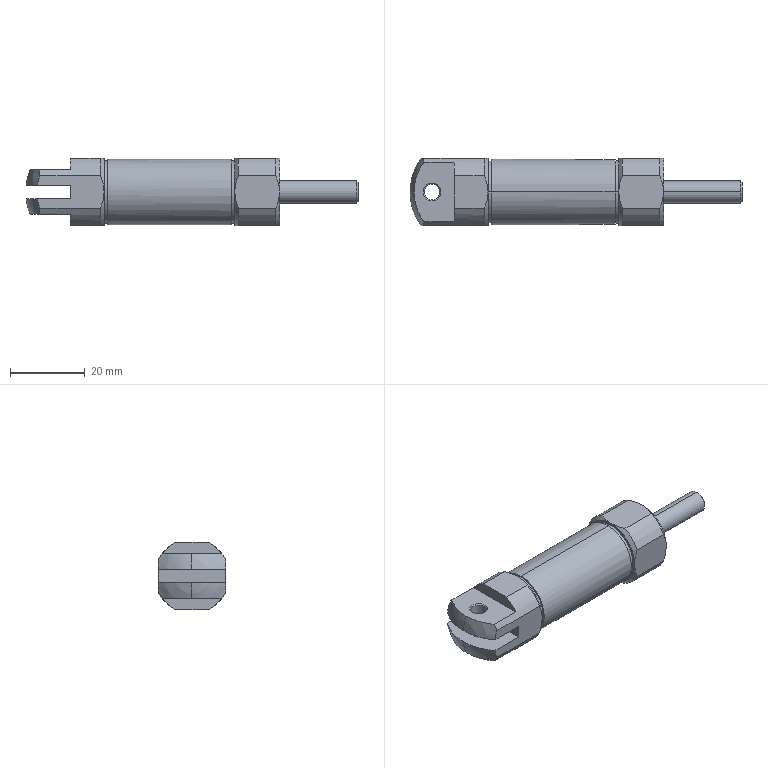Part | STEP file | 101000005927 | 2 solids | 78 faces | box 88.898 x 18 x 18 mm | volume 15835 mm3 | cylinder 28 | plane 24 | cone 22 | sphere 4 | commonest cylinder face diameters 4.2 x10 20 x8 6 x4 16.7 x4 17.5 x2